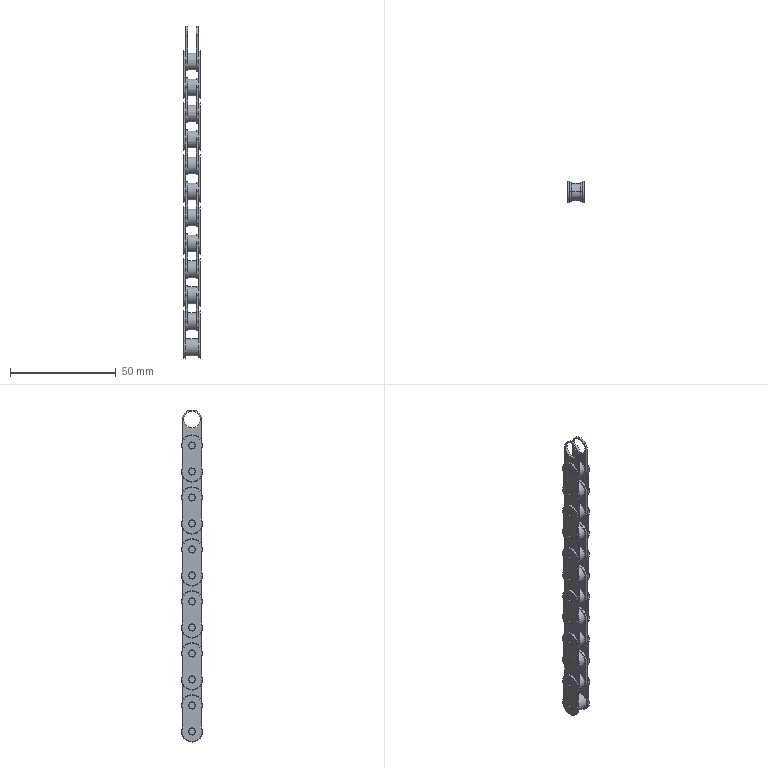Part | STEP file | 6 Chain Links v2 | 6 solids | 396 faces | box 8 x 10 x 157.1 mm | volume 6633 mm3 | cylinder 192 | plane 120 | torus 84 | commonest cylinder face diameters 3 x48 8 x48 9 x36 10 x36 0.4 x24